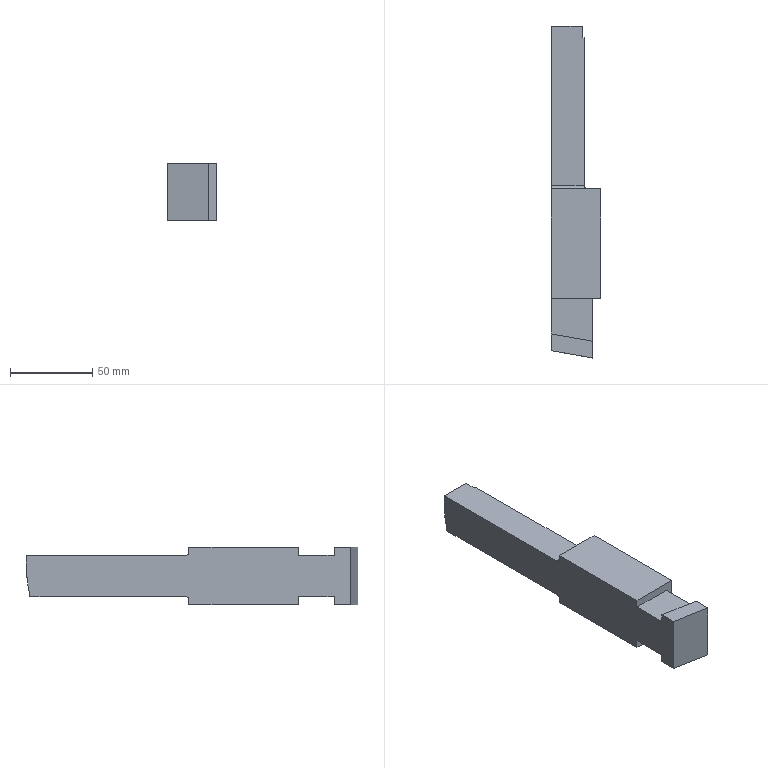Part | STEP file | solid 34 | 1 solid | 34 faces | box 30 x 202.213 x 35 mm | volume 142973 mm3 | plane 20 | spline 7 | cylinder 6 | torus 1 | commonest cylinder face diameters 4 x3 0.502 x1 1.206 x1 6.03 x1